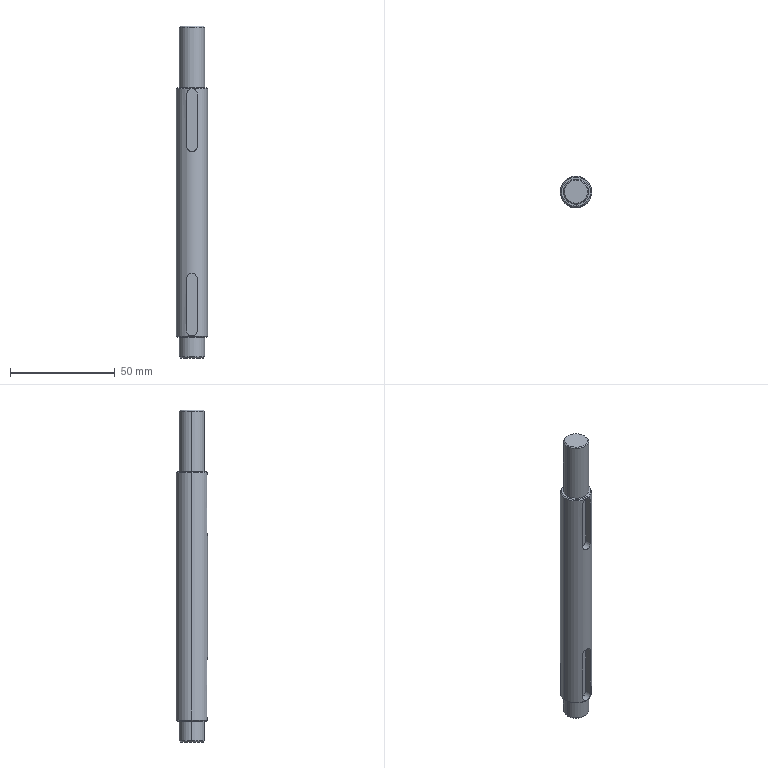Part | SolidWorks | features ICE 3, Chamfer 2, Extrusion 1 | 1 solid | 30 faces | box 15 x 15 x 158.5 mm | volume 24503 mm3 | cylinder 12 | plane 10 | cone 8 | commonest cylinder face diameters 5 x6 12 x4 15 x2
STEP:
#1=CARTESIAN_POINT('',(2.5,-7.071,-120.5));
#2=VERTEX_POINT('',#1);
#3=CARTESIAN_POINT('',(0.,-7.5,-118.));
#4=VERTEX_POINT('',#3);
#5=CARTESIAN_POINT('',(2.5,-7.071,-120.5));
#6=CARTESIAN_POINT('',(2.5,-7.071,-120.335));
#7=CARTESIAN_POINT('',(2.484,-7.077,-120.172));
#8=CARTESIAN_POINT('',(2.419,-7.099,-119.849));
#9=CARTESIAN_POINT('',(2.371,-7.116,-119.69));
#10=CARTESIAN_POINT('',(2.183,-7.177,-119.238));
#11=CARTESIAN_POINT('',(1.997,-7.233,-118.962));
#12=CARTESIAN_POINT('',(1.654,-7.316,-118.618));
#13=CARTESIAN_POINT('',(1.526,-7.344,-118.513));
#14=CARTESIAN_POINT('',(1.256,-7.395,-118.332));
#15=CARTESIAN_POINT('',(1.113,-7.419,-118.255));
#16=CARTESIAN_POINT('',(0.8106,-7.458,-118.129));
#17=CARTESIAN_POINT('',(0.6511,-7.473,-118.081));
#18=CARTESIAN_POINT('',(0.33,-7.494,-118.016));
#19=CARTESIAN_POINT('',(0.1664,-7.5,-118.));
#20=CARTESIAN_POINT('',(0.,-7.5,-118.));
#21=B_SPLINE_CURVE_WITH_KNOTS('',3,(#5,#6,#7,#8,#9,#10,#11,#12,#13,#14,#15,#16,#17,#18,#19,#20),.UNSPECIFIED.,.F.,.F.,(4,2,2,2,2,2,2,4),(0.01181,0.0123,0.01279,0.01378,0.01427,0.01476,0.01525,0.01574),.UNSPECIFIED.);
#22=EDGE_CURVE('',#2,#4,#21,.T.);
#23=ORIENTED_EDGE('',*,*,#22,.T.);
#24=CARTESIAN_POINT('',(0.,-4.,-118.));
#25=VERTEX_POINT('',#24);
#26=CARTESIAN_POINT('',(0.,-52.,-118.));
#27=DIRECTION('',(0.,1.,0.));
#28=VECTOR('',#27,1000.);
#29=LINE('',#26,#28);
#30=EDGE_CURVE('',#4,#25,#29,.T.);
#31=ORIENTED_EDGE('',*,*,#30,.T.);
#32=CARTESIAN_POINT('',(2.5,-4.,-120.5));
#33=VERTEX_POINT('',#32);
#34=CARTESIAN_POINT('',(0.,-4.,-120.5));
#35=DIRECTION('',(0.,1.,0.));
#36=DIRECTION('',(0.,0.,1.));
#37=AXIS2_PLACEMENT_3D('',#34,#35,#36);
#38=CIRCLE('',#37,2.5);
#39=EDGE_CURVE('',#25,#33,#38,.T.);
#40=ORIENTED_EDGE('',*,*,#39,.T.);
#41=CARTESIAN_POINT('',(2.5,-52.,-120.5));
#42=DIRECTION('',(0.,1.,0.));
#43=VECTOR('',#42,1000.);
#44=LINE('',#41,#43);
#45=EDGE_CURVE('',#2,#33,#44,.T.);
#46=ORIENTED_EDGE('',*,*,#45,.F.);
#47=EDGE_LOOP('',(#23,#31,#40,#46));
#48=FACE_OUTER_BOUND('',#47,.T.);
#49=CARTESIAN_POINT('',(0.,-52.,-120.5));
#50=DIRECTION('',(0.,1.,0.));
#51=DIRECTION('',(0.,0.,1.));
#52=AXIS2_PLACEMENT_3D('',#49,#50,#51);
#53=CYLINDRICAL_SURFACE('',#52,2.5);
#54=ADVANCED_FACE('',(#48),#53,.F.);
#55=CARTESIAN_POINT('',(2.5,-7.071,-32.5));
#56=VERTEX_POINT('',#55);
#57=CARTESIAN_POINT('',(0.,-7.5,-30.));
#58=VERTEX_POINT('',#57);
#59=CARTESIAN_POINT('',(2.5,-7.071,-32.5));
#60=CARTESIAN_POINT('',(2.5,-7.071,-32.335));
#61=CARTESIAN_POINT('',(2.484,-7.077,-32.172));
#62=CARTESIAN_POINT('',(2.419,-7.099,-31.849));
#63=CARTESIAN_POINT('',(2.371,-7.116,-31.69));
#64=CARTESIAN_POINT('',(2.183,-7.177,-31.238));
#65=CARTESIAN_POINT('',(1.997,-7.233,-30.962));
#66=CARTESIAN_POINT('',(1.654,-7.316,-30.618));
#67=CARTESIAN_POINT('',(1.526,-7.344,-30.513));
#68=CARTESIAN_POINT('',(1.256,-7.395,-30.332));
#69=CARTESIAN_POINT('',(1.113,-7.419,-30.255));
#70=CARTESIAN_POINT('',(0.8106,-7.458,-30.129));
#71=CARTESIAN_POINT('',(0.6511,-7.473,-30.081));
#72=CARTESIAN_POINT('',(0.33,-7.494,-30.016));
#73=CARTESIAN_POINT('',(0.1664,-7.5,-30.));
#74=CARTESIAN_POINT('',(0.,-7.5,-30.));
#75=B_SPLINE_CURVE_WITH_KNOTS('',3,(#59,#60,#61,#62,#63,#64,#65,#66,#67,#68,#69,#70,#71,#72,#73,#74),.UNSPECIFIED.,.F.,.F.,(4,2,2,2,2,2,2,4),(0.01181,0.0123,0.01279,0.01378,0.01427,0.01476,0.01525,0.01574),.UNSPECIFIED.);
#76=EDGE_CURVE('',#56,#58,#75,.T.);
#77=ORIENTED_EDGE('',*,*,#76,.T.);
#78=CARTESIAN_POINT('',(0.,-4.,-30.));
#79=VERTEX_POINT('',#78);
#80=CARTESIAN_POINT('',(0.,-52.,-30.));
#81=DIRECTION('',(0.,1.,0.));
#82=VECTOR('',#81,1000.);
#83=LINE('',#80,#82);
#84=EDGE_CURVE('',#58,#79,#83,.T.);
#85=ORIENTED_EDGE('',*,*,#84,.T.);
#86=CARTESIAN_POINT('',(2.5,-4.,-32.5));
#87=VERTEX_POINT('',#86);
#88=CARTESIAN_POINT('',(0.,-4.,-32.5));
#89=DIRECTION('',(0.,1.,0.));
#90=DIRECTION('',(0.,0.,1.));
#91=AXIS2_PLACEMENT_3D('',#88,#89,#90);
#92=CIRCLE('',#91,2.5);
#93=EDGE_CURVE('',#79,#87,#92,.T.);
#94=ORIENTED_EDGE('',*,*,#93,.T.);
#95=CARTESIAN_POINT('',(2.5,-52.,-32.5));
#96=DIRECTION('',(0.,1.,0.));
#97=VECTOR('',#96,1000.);
#98=LINE('',#95,#97);
#99=EDGE_CURVE('',#56,#87,#98,.T.);
#100=ORIENTED_EDGE('',*,*,#99,.F.);
#101=EDGE_LOOP('',(#77,#85,#94,#100));
#102=FACE_OUTER_BOUND('',#101,.T.);
#103=CARTESIAN_POINT('',(0.,-52.,-32.5));
#104=DIRECTION('',(0.,1.,0.));
#105=DIRECTION('',(0.,0.,1.));
#106=AXIS2_PLACEMENT_3D('',#103,#104,#105);
#107=CYLINDRICAL_SURFACE('',#106,2.5);
#108=ADVANCED_FACE('',(#102),#107,.F.);
#109=CARTESIAN_POINT('',(-5.5,0.,-158.5));
#110=VERTEX_POINT('',#109);
#111=CARTESIAN_POINT('',(5.5,0.,-158.5));
#112=VERTEX_POINT('',#111);
#113=CARTESIAN_POINT('',(0.,0.,-158.5));
#114=DIRECTION('',(0.,0.,-1.));
#115=DIRECTION('',(1.,0.,0.));
#116=AXIS2_PLACEMENT_3D('',#113,#114,#115);
#117=CIRCLE('',#116,5.5);
#118=EDGE_CURVE('',#110,#112,#117,.T.);
#119=ORIENTED_EDGE('',*,*,#118,.F.);
#120=CARTESIAN_POINT('',(-6.,0.,-158.));
#121=VERTEX_POINT('',#120);
#122=CARTESIAN_POINT('',(-5.5,0.,-158.5));
#123=DIRECTION('',(-0.7071,0.,0.7071));
#124=VECTOR('',#123,1000.);
#125=LINE('',#122,#124);
#126=EDGE_CURVE('',#110,#121,#125,.T.);
#127=ORIENTED_EDGE('',*,*,#126,.T.);
#128=CARTESIAN_POINT('',(6.,0.,-158.));
#129=VERTEX_POINT('',#128);
#130=CARTESIAN_POINT('',(0.,0.,-158.));
#131=DIRECTION('',(0.,0.,1.));
#132=DIRECTION('',(1.,0.,0.));
#133=AXIS2_PLACEMENT_3D('',#130,#131,#132);
#134=CIRCLE('',#133,6.);
#135=EDGE_CURVE('',#129,#121,#134,.T.);
#136=ORIENTED_EDGE('',*,*,#135,.F.);
#137=CARTESIAN_POINT('',(5.5,0.,-158.5));
#138=DIRECTION('',(0.7071,0.,0.7071));
#139=VECTOR('',#138,1000.);
#140=LINE('',#137,#139);
#141=EDGE_CURVE('',#112,#129,#140,.T.);
#142=ORIENTED_EDGE('',*,*,#141,.F.);
#143=EDGE_LOOP('',(#119,#127,#136,#142));
#144=FACE_OUTER_BOUND('',#143,.T.);
#145=CARTESIAN_POINT('',(0.,0.,-158.5));
#146=DIRECTION('',(0.,0.,1.));
#147=DIRECTION('',(1.,0.,0.));
#148=AXIS2_PLACEMENT_3D('',#145,#146,#147);
#149=CONICAL_SURFACE('',#148,5.5,0.7854);
#150=ADVANCED_FACE('',(#144),#149,.T.);
#151=CARTESIAN_POINT('',(-7.,0.,-148.5));
#152=VERTEX_POINT('',#151);
#153=CARTESIAN_POINT('',(7.,0.,-148.5));
#154=VERTEX_POINT('',#153);
#155=CARTESIAN_POINT('',(0.,0.,-148.5));
#156=DIRECTION('',(0.,0.,-1.));
#157=DIRECTION('',(-1.,0.,0.));
#158=AXIS2_PLACEMENT_3D('',#155,#156,#157);
#159=CIRCLE('',#158,7.);
#160=EDGE_CURVE('',#152,#154,#159,.T.);
#161=ORIENTED_EDGE('',*,*,#160,.F.);
#162=CARTESIAN_POINT('',(-7.5,0.,-148.));
#163=VERTEX_POINT('',#162);
#164=CARTESIAN_POINT('',(-7.5,0.,-148.));
#165=DIRECTION('',(-0.7071,0.,0.7071));
#166=VECTOR('',#165,1000.);
#167=LINE('',#164,#166);
#168=EDGE_CURVE('',#152,#163,#167,.T.);
#169=ORIENTED_EDGE('',*,*,#168,.T.);
#170=CARTESIAN_POINT('',(7.5,0.,-148.));
#171=VERTEX_POINT('',#170);
#172=CARTESIAN_POINT('',(0.,0.,-148.));
#173=DIRECTION('',(0.,0.,1.));
#174=DIRECTION('',(-1.,0.,0.));
#175=AXIS2_PLACEMENT_3D('',#172,#173,#174);
#176=CIRCLE('',#175,7.5);
#177=EDGE_CURVE('',#171,#163,#176,.T.);
#178=ORIENTED_EDGE('',*,*,#177,.F.);
#179=CARTESIAN_POINT('',(7.5,0.,-148.));
#180=DIRECTION('',(0.7071,0.,0.7071));
#181=VECTOR('',#180,1000.);
#182=LINE('',#179,#181);
#183=EDGE_CURVE('',#154,#171,#182,.T.);
#184=ORIENTED_EDGE('',*,*,#183,.F.);
#185=EDGE_LOOP('',(#161,#169,#178,#184));
#186=FACE_OUTER_BOUND('',#185,.T.);
#187=CARTESIAN_POINT('',(0.,0.,-148.));
#188=DIRECTION('',(0.,0.,1.));
#189=DIRECTION('',(1.,0.,0.));
#190=AXIS2_PLACEMENT_3D('',#187,#188,#189);
#191=CONICAL_SURFACE('',#190,7.5,0.7854);
#192=ADVANCED_FACE('',(#186),#191,.T.);
#193=CARTESIAN_POINT('',(-6.,0.,-148.5));
#194=VERTEX_POINT('',#193);
#195=CARTESIAN_POINT('',(6.,0.,-148.5));
#196=VERTEX_POINT('',#195);
#197=CARTESIAN_POINT('',(0.,0.,-148.5));
#198=DIRECTION('',(0.,0.,-1.));
#199=DIRECTION('',(-1.,0.,0.));
#200=AXIS2_PLACEMENT_3D('',#197,#198,#199);
#201=CIRCLE('',#200,6.);
#202=EDGE_CURVE('',#194,#196,#201,.T.);
#203=ORIENTED_EDGE('',*,*,#202,.T.);
#204=CARTESIAN_POINT('',(6.,0.,-148.5));
#205=DIRECTION('',(0.,0.,-1.));
#206=VECTOR('',#205,1000.);
#207=LINE('',#204,#206);
#208=EDGE_CURVE('',#196,#129,#207,.T.);
#209=ORIENTED_EDGE('',*,*,#208,.T.);
#210=ORIENTED_EDGE('',*,*,#135,.T.);
#211=CARTESIAN_POINT('',(-6.,0.,-148.5));
#212=DIRECTION('',(0.,0.,-1.));
#213=VECTOR('',#212,1000.);
#214=LINE('',#211,#213);
#215=EDGE_CURVE('',#194,#121,#214,.T.);
#216=ORIENTED_EDGE('',*,*,#215,.F.);
#217=EDGE_LOOP('',(#203,#209,#210,#216));
#218=FACE_OUTER_BOUND('',#217,.T.);
#219=CARTESIAN_POINT('',(0.,0.,-148.5));
#220=DIRECTION('',(0.,0.,-1.));
#221=DIRECTION('',(-1.,0.,0.));
#222=AXIS2_PLACEMENT_3D('',#219,#220,#221);
#223=CYLINDRICAL_SURFACE('',#222,6.);
#224=ADVANCED_FACE('',(#218),#223,.T.);
#225=CARTESIAN_POINT('',(5.5,0.,0.));
#226=VERTEX_POINT('',#225);
#227=CARTESIAN_POINT('',(-5.5,0.,0.));
#228=VERTEX_POINT('',#227);
#229=CARTESIAN_POINT('',(0.,0.,0.));
#230=DIRECTION('',(0.,0.,1.));
#231=DIRECTION('',(1.,0.,0.));
#232=AXIS2_PLACEMENT_3D('',#229,#230,#231);
#233=CIRCLE('',#232,5.5);
#234=EDGE_CURVE('',#226,#228,#233,.T.);
#235=ORIENTED_EDGE('',*,*,#234,.F.);
#236=CARTESIAN_POINT('',(6.,0.,-0.5));
#237=VERTEX_POINT('',#236);
#238=CARTESIAN_POINT('',(5.5,0.,0.));
#239=DIRECTION('',(0.7071,0.,-0.7071));
#240=VECTOR('',#239,1000.);
#241=LINE('',#238,#240);
#242=EDGE_CURVE('',#226,#237,#241,.T.);
#243=ORIENTED_EDGE('',*,*,#242,.T.);
#244=CARTESIAN_POINT('',(-6.,0.,-0.5));
#245=VERTEX_POINT('',#244);
#246=CARTESIAN_POINT('',(0.,0.,-0.5));
#247=DIRECTION('',(0.,0.,-1.));
#248=DIRECTION('',(1.,0.,0.));
#249=AXIS2_PLACEMENT_3D('',#246,#247,#248);
#250=CIRCLE('',#249,6.);
#251=EDGE_CURVE('',#245,#237,#250,.T.);
#252=ORIENTED_EDGE('',*,*,#251,.F.);
#253=CARTESIAN_POINT('',(-5.5,0.,0.));
#254=DIRECTION('',(-0.7071,0.,-0.7071));
#255=VECTOR('',#254,1000.);
#256=LINE('',#253,#255);
#257=EDGE_CURVE('',#228,#245,#256,.T.);
#258=ORIENTED_EDGE('',*,*,#257,.F.);
#259=EDGE_LOOP('',(#235,#243,#252,#258));
#260=FACE_OUTER_BOUND('',#259,.T.);
#261=CARTESIAN_POINT('',(0.,0.,0.));
#262=DIRECTION('',(0.,0.,-1.));
#263=DIRECTION('',(-1.,0.,0.));
#264=AXIS2_PLACEMENT_3D('',#261,#262,#263);
#265=CONICAL_SURFACE('',#264,5.5,0.7854);
#266=ADVANCED_FACE('',(#260),#265,.T.);
#267=CARTESIAN_POINT('',(7.,0.,-29.5));
#268=VERTEX_POINT('',#267);
#269=CARTESIAN_POINT('',(-7.,0.,-29.5));
#270=VERTEX_POINT('',#269);
#271=CARTESIAN_POINT('',(0.,0.,-29.5));
#272=DIRECTION('',(0.,0.,1.));
#273=DIRECTION('',(1.,0.,0.));
#274=AXIS2_PLACEMENT_3D('',#271,#272,#273);
#275=CIRCLE('',#274,7.);
#276=EDGE_CURVE('',#268,#270,#275,.T.);
#277=ORIENTED_EDGE('',*,*,#276,.F.);
#278=CARTESIAN_POINT('',(7.5,0.,-30.));
#279=VERTEX_POINT('',#278);
#280=CARTESIAN_POINT('',(7.5,0.,-30.));
#281=DIRECTION('',(0.7071,0.,-0.7071));
#282=VECTOR('',#281,1000.);
#283=LINE('',#280,#282);
#284=EDGE_CURVE('',#268,#279,#283,.T.);
#285=ORIENTED_EDGE('',*,*,#284,.T.);
#286=CARTESIAN_POINT('',(-7.5,0.,-30.));
#287=VERTEX_POINT('',#286);
#288=CARTESIAN_POINT('',(0.,0.,-30.));
#289=DIRECTION('',(0.,0.,-1.));
#290=DIRECTION('',(1.,0.,0.));
#291=AXIS2_PLACEMENT_3D('',#288,#289,#290);
#292=CIRCLE('',#291,7.5);
#293=EDGE_CURVE('',#287,#279,#292,.T.);
#294=ORIENTED_EDGE('',*,*,#293,.F.);
#295=CARTESIAN_POINT('',(-7.5,0.,-30.));
#296=DIRECTION('',(-0.7071,0.,-0.7071));
#297=VECTOR('',#296,1000.);
#298=LINE('',#295,#297);
#299=EDGE_CURVE('',#270,#287,#298,.T.);
#300=ORIENTED_EDGE('',*,*,#299,.F.);
#301=EDGE_LOOP('',(#277,#285,#294,#300));
#302=FACE_OUTER_BOUND('',#301,.T.);
#303=CARTESIAN_POINT('',(0.,0.,-30.));
#304=DIRECTION('',(0.,0.,-1.));
#305=DIRECTION('',(-1.,0.,0.));
#306=AXIS2_PLACEMENT_3D('',#303,#304,#305);
#307=CONICAL_SURFACE('',#306,7.5,0.7854);
#308=ADVANCED_FACE('',(#302),#307,.T.);
#309=CARTESIAN_POINT('',(6.,0.,-29.5));
#310=VERTEX_POINT('',#309);
#311=CARTESIAN_POINT('',(-6.,0.,-29.5));
#312=VERTEX_POINT('',#311);
#313=CARTESIAN_POINT('',(0.,0.,-29.5));
#314=DIRECTION('',(0.,0.,1.));
#315=DIRECTION('',(1.,0.,0.));
#316=AXIS2_PLACEMENT_3D('',#313,#314,#315);
#317=CIRCLE('',#316,6.);
#318=EDGE_CURVE('',#310,#312,#317,.T.);
#319=ORIENTED_EDGE('',*,*,#318,.T.);
#320=CARTESIAN_POINT('',(-6.,0.,-29.5));
#321=DIRECTION('',(0.,0.,1.));
#322=VECTOR('',#321,1000.);
#323=LINE('',#320,#322);
#324=EDGE_CURVE('',#312,#245,#323,.T.);
#325=ORIENTED_EDGE('',*,*,#324,.T.);
#326=ORIENTED_EDGE('',*,*,#251,.T.);
#327=CARTESIAN_POINT('',(6.,0.,-29.5));
#328=DIRECTION('',(0.,0.,1.));
#329=VECTOR('',#328,1000.);
#330=LINE('',#327,#329);
#331=EDGE_CURVE('',#310,#237,#330,.T.);
#332=ORIENTED_EDGE('',*,*,#331,.F.);
#333=EDGE_LOOP('',(#319,#325,#326,#332));
#334=FACE_OUTER_BOUND('',#333,.T.);
#335=CARTESIAN_POINT('',(0.,0.,-29.5));
#336=DIRECTION('',(0.,0.,1.));
#337=DIRECTION('',(1.,0.,0.));
#338=AXIS2_PLACEMENT_3D('',#335,#336,#337);
#339=CYLINDRICAL_SURFACE('',#338,6.);
#340=ADVANCED_FACE('',(#334),#339,.T.);
#341=ORIENTED_EDGE('',*,*,#177,.T.);
#342=CARTESIAN_POINT('',(-7.5,0.,-158.5));
#343=DIRECTION('',(0.,0.,1.));
#344=VECTOR('',#343,1000.);
#345=LINE('',#342,#344);
#346=EDGE_CURVE('',#163,#287,#345,.T.);
#347=ORIENTED_EDGE('',*,*,#346,.T.);
#348=ORIENTED_EDGE('',*,*,#293,.T.);
#349=CARTESIAN_POINT('',(7.5,0.,-158.5));
#350=DIRECTION('',(0.,0.,1.));
#351=VECTOR('',#350,1000.);
#352=LINE('',#349,#351);
#353=EDGE_CURVE('',#171,#279,#352,.T.);
#354=ORIENTED_EDGE('',*,*,#353,.F.);
#355=EDGE_LOOP('',(#341,#347,#348,#354));
#356=FACE_OUTER_BOUND('',#355,.T.);
#357=CARTESIAN_POINT('',(0.,0.,-158.5));
#358=DIRECTION('',(0.,0.,1.));
#359=DIRECTION('',(1.,0.,0.));
#360=AXIS2_PLACEMENT_3D('',#357,#358,#359);
#361=CYLINDRICAL_SURFACE('',#360,7.5);
#362=ADVANCED_FACE('',(#356),#361,.T.);
#363=ORIENTED_EDGE('',*,*,#346,.F.);
#364=CARTESIAN_POINT('',(0.,-7.5,-148.));
#365=VERTEX_POINT('',#364);
#366=CARTESIAN_POINT('',(0.,0.,-148.));
#367=DIRECTION('',(0.,0.,1.));
#368=DIRECTION('',(-1.,0.,0.));
#369=AXIS2_PLACEMENT_3D('',#366,#367,#368);
#370=CIRCLE('',#369,7.5);
#371=EDGE_CURVE('',#163,#365,#370,.T.);
#372=ORIENTED_EDGE('',*,*,#371,.T.);
#373=CARTESIAN_POINT('',(-2.5,-7.071,-145.5));
#374=VERTEX_POINT('',#373);
#375=CARTESIAN_POINT('',(-2.5,-7.071,-145.5));
#376=CARTESIAN_POINT('',(-2.5,-7.071,-145.664));
#377=CARTESIAN_POINT('',(-2.483,-7.077,-145.831));
#378=CARTESIAN_POINT('',(-2.419,-7.099,-146.153));
#379=CARTESIAN_POINT('',(-2.371,-7.116,-146.309));
#380=CARTESIAN_POINT('',(-2.244,-7.157,-146.613));
#381=CARTESIAN_POINT('',(-2.167,-7.181,-146.757));
#382=CARTESIAN_POINT('',(-1.986,-7.233,-147.027));
#383=CARTESIAN_POINT('',(-1.882,-7.261,-147.154));
#384=CARTESIAN_POINT('',(-1.652,-7.317,-147.384));
#385=CARTESIAN_POINT('',(-1.527,-7.344,-147.486));
#386=CARTESIAN_POINT('',(-1.257,-7.395,-147.667));
#387=CARTESIAN_POINT('',(-1.11,-7.419,-147.746));
#388=CARTESIAN_POINT('',(-0.8092,-7.458,-147.871));
#389=CARTESIAN_POINT('',(-0.6532,-7.473,-147.919));
#390=CARTESIAN_POINT('',(-0.3296,-7.495,-147.984));
#391=CARTESIAN_POINT('',(-0.1639,-7.5,-148.));
#392=CARTESIAN_POINT('',(0.,-7.5,-148.));
#393=B_SPLINE_CURVE_WITH_KNOTS('',3,(#375,#376,#377,#378,#379,#380,#381,#382,#383,#384,#385,#386,#387,#388,#389,#390,#391,#392),.UNSPECIFIED.,.F.,.F.,(4,2,2,2,2,2,2,2,4),(0.003938,0.00443,0.004921,0.005413,0.005905,0.006397,0.006889,0.007381,0.007873),.UNSPECIFIED.);
#394=EDGE_CURVE('',#374,#365,#393,.T.);
#395=ORIENTED_EDGE('',*,*,#394,.F.);
#396=CARTESIAN_POINT('',(-2.5,-7.071,-120.5));
#397=VERTEX_POINT('',#396);
#398=CARTESIAN_POINT('',(-2.5,-7.071,-158.5));
#399=DIRECTION('',(0.,0.,-1.));
#400=VECTOR('',#399,1000.);
#401=LINE('',#398,#400);
#402=EDGE_CURVE('',#397,#374,#401,.T.);
#403=ORIENTED_EDGE('',*,*,#402,.F.);
#404=CARTESIAN_POINT('',(0.,-7.5,-118.));
#405=CARTESIAN_POINT('',(-0.1665,-7.5,-118.));
#406=CARTESIAN_POINT('',(-0.33,-7.494,-118.016));
#407=CARTESIAN_POINT('',(-0.6513,-7.473,-118.081));
#408=CARTESIAN_POINT('',(-0.8108,-7.458,-118.129));
#409=CARTESIAN_POINT('',(-1.113,-7.418,-118.256));
#410=CARTESIAN_POINT('',(-1.256,-7.395,-118.333));
#411=CARTESIAN_POINT('',(-1.527,-7.344,-118.514));
#412=CARTESIAN_POINT('',(-1.655,-7.316,-118.619));
#413=CARTESIAN_POINT('',(-1.998,-7.233,-118.963));
#414=CARTESIAN_POINT('',(-2.183,-7.176,-119.24));
#415=CARTESIAN_POINT('',(-2.371,-7.116,-119.69));
#416=CARTESIAN_POINT('',(-2.419,-7.099,-119.849));
#417=CARTESIAN_POINT('',(-2.484,-7.077,-120.172));
#418=CARTESIAN_POINT('',(-2.5,-7.071,-120.336));
#419=CARTESIAN_POINT('',(-2.5,-7.071,-120.5));
#420=B_SPLINE_CURVE_WITH_KNOTS('',3,(#404,#405,#406,#407,#408,#409,#410,#411,#412,#413,#414,#415,#416,#417,#418,#419),.UNSPECIFIED.,.F.,.F.,(4,2,2,2,2,2,2,4),(0.,0.0004922,0.0009844,0.001477,0.001969,0.002953,0.003445,0.003938),.UNSPECIFIED.);
#421=EDGE_CURVE('',#4,#397,#420,.T.);
#422=ORIENTED_EDGE('',*,*,#421,.F.);
#423=ORIENTED_EDGE('',*,*,#22,.F.);
#424=CARTESIAN_POINT('',(2.5,-7.071,-145.5));
#425=VERTEX_POINT('',#424);
#426=CARTESIAN_POINT('',(2.5,-7.071,-158.5));
#427=DIRECTION('',(0.,0.,1.));
#428=VECTOR('',#427,1000.);
#429=LINE('',#426,#428);
#430=EDGE_CURVE('',#425,#2,#429,.T.);
#431=ORIENTED_EDGE('',*,*,#430,.F.);
#432=CARTESIAN_POINT('',(0.,-7.5,-148.));
#433=CARTESIAN_POINT('',(0.1639,-7.5,-148.));
#434=CARTESIAN_POINT('',(0.329,-7.495,-147.984));
#435=CARTESIAN_POINT('',(0.6533,-7.473,-147.919));
#436=CARTESIAN_POINT('',(0.8096,-7.458,-147.871));
#437=CARTESIAN_POINT('',(1.111,-7.419,-147.745));
#438=CARTESIAN_POINT('',(1.258,-7.395,-147.667));
#439=CARTESIAN_POINT('',(1.527,-7.344,-147.486));
#440=CARTESIAN_POINT('',(1.653,-7.317,-147.383));
#441=CARTESIAN_POINT('',(1.999,-7.233,-147.037));
#442=CARTESIAN_POINT('',(2.182,-7.177,-146.764));
#443=CARTESIAN_POINT('',(2.371,-7.116,-146.308));
#444=CARTESIAN_POINT('',(2.419,-7.099,-146.152));
#445=CARTESIAN_POINT('',(2.483,-7.077,-145.831));
#446=CARTESIAN_POINT('',(2.5,-7.071,-145.665));
#447=CARTESIAN_POINT('',(2.5,-7.071,-145.5));
#448=B_SPLINE_CURVE_WITH_KNOTS('',3,(#432,#433,#434,#435,#436,#437,#438,#439,#440,#441,#442,#443,#444,#445,#446,#447),.UNSPECIFIED.,.F.,.F.,(4,2,2,2,2,2,2,4),(0.007873,0.008365,0.008857,0.009349,0.00984,0.01082,0.01132,0.01181),.UNSPECIFIED.);
#449=EDGE_CURVE('',#365,#425,#448,.T.);
#450=ORIENTED_EDGE('',*,*,#449,.F.);
#451=CARTESIAN_POINT('',(0.,0.,-148.));
#452=DIRECTION('',(0.,0.,1.));
#453=DIRECTION('',(-1.,0.,0.));
#454=AXIS2_PLACEMENT_3D('',#451,#452,#453);
#455=CIRCLE('',#454,7.5);
#456=EDGE_CURVE('',#365,#171,#455,.T.);
#457=ORIENTED_EDGE('',*,*,#456,.T.);
#458=ORIENTED_EDGE('',*,*,#353,.T.);
#459=CARTESIAN_POINT('',(0.,0.,-30.));
#460=DIRECTION('',(0.,0.,-1.));
#461=DIRECTION('',(1.,0.,0.));
#462=AXIS2_PLACEMENT_3D('',#459,#460,#461);
#463=CIRCLE('',#462,7.5);
#464=EDGE_CURVE('',#279,#58,#463,.T.);
#465=ORIENTED_EDGE('',*,*,#464,.T.);
#466=ORIENTED_EDGE('',*,*,#76,.F.);
#467=CARTESIAN_POINT('',(2.5,-7.071,-57.5));
#468=VERTEX_POINT('',#467);
#469=CARTESIAN_POINT('',(2.5,-7.071,-158.5));
#470=DIRECTION('',(0.,0.,1.));
#471=VECTOR('',#470,1000.);
#472=LINE('',#469,#471);
#473=EDGE_CURVE('',#468,#56,#472,.T.);
#474=ORIENTED_EDGE('',*,*,#473,.F.);
#475=CARTESIAN_POINT('',(-2.5,-7.071,-57.5));
#476=VERTEX_POINT('',#475);
#477=CARTESIAN_POINT('',(-2.5,-7.071,-57.5));
#478=CARTESIAN_POINT('',(-2.5,-7.071,-57.664));
#479=CARTESIAN_POINT('',(-2.483,-7.077,-57.831));
#480=CARTESIAN_POINT('',(-2.419,-7.099,-58.153));
#481=CARTESIAN_POINT('',(-2.371,-7.116,-58.309));
#482=CARTESIAN_POINT('',(-2.244,-7.157,-58.613));
#483=CARTESIAN_POINT('',(-2.167,-7.181,-58.757));
#484=CARTESIAN_POINT('',(-1.986,-7.233,-59.027));
#485=CARTESIAN_POINT('',(-1.882,-7.261,-59.154));
#486=CARTESIAN_POINT('',(-1.652,-7.317,-59.384));
#487=CARTESIAN_POINT('',(-1.527,-7.344,-59.486));
#488=CARTESIAN_POINT('',(-1.257,-7.395,-59.667));
#489=CARTESIAN_POINT('',(-1.11,-7.419,-59.746));
#490=CARTESIAN_POINT('',(-0.8093,-7.458,-59.871));
#491=CARTESIAN_POINT('',(-0.6533,-7.473,-59.919));
#492=CARTESIAN_POINT('',(-0.3296,-7.495,-59.984));
#493=CARTESIAN_POINT('',(-0.164,-7.5,-60.));
#494=CARTESIAN_POINT('',(0.1639,-7.5,-60.));
#495=CARTESIAN_POINT('',(0.329,-7.495,-59.984));
#496=CARTESIAN_POINT('',(0.6533,-7.473,-59.919));
#497=CARTESIAN_POINT('',(0.8096,-7.458,-59.871));
#498=CARTESIAN_POINT('',(1.111,-7.419,-59.745));
#499=CARTESIAN_POINT('',(1.257,-7.395,-59.667));
#500=CARTESIAN_POINT('',(1.527,-7.344,-59.486));
#501=CARTESIAN_POINT('',(1.653,-7.317,-59.383));
#502=CARTESIAN_POINT('',(1.999,-7.233,-59.037));
#503=CARTESIAN_POINT('',(2.182,-7.177,-58.764));
#504=CARTESIAN_POINT('',(2.371,-7.116,-58.308));
#505=CARTESIAN_POINT('',(2.419,-7.099,-58.152));
#506=CARTESIAN_POINT('',(2.483,-7.077,-57.831));
#507=CARTESIAN_POINT('',(2.5,-7.071,-57.665));
#508=CARTESIAN_POINT('',(2.5,-7.071,-57.5));
#509=B_SPLINE_CURVE_WITH_KNOTS('',3,(#477,#478,#479,#480,#481,#482,#483,#484,#485,#486,#487,#488,#489,#490,#491,#492,#493,#494,#495,#496,#497,#498,#499,#500,#501,#502,#503,#504,#505,#506,#507,#508),.UNSPECIFIED.,.F.,.F.,(4,2,2,2,2,2,2,2,2,2,2,2,2,2,2,4),(0.003938,0.00443,0.004921,0.005413,0.005905,0.006397,0.006889,0.007381,0.007873,0.008365,0.008857,0.009349,0.00984,0.01082,0.01132,0.01181),.UNSPECIFIED.);
#510=EDGE_CURVE('',#476,#468,#509,.T.);
#511=ORIENTED_EDGE('',*,*,#510,.F.);
#512=CARTESIAN_POINT('',(-2.5,-7.071,-32.5));
#513=VERTEX_POINT('',#512);
#514=CARTESIAN_POINT('',(-2.5,-7.071,-158.5));
#515=DIRECTION('',(0.,0.,-1.));
#516=VECTOR('',#515,1000.);
#517=LINE('',#514,#516);
#518=EDGE_CURVE('',#513,#476,#517,.T.);
#519=ORIENTED_EDGE('',*,*,#518,.F.);
#520=CARTESIAN_POINT('',(0.,-7.5,-30.));
#521=CARTESIAN_POINT('',(-0.1665,-7.5,-30.));
#522=CARTESIAN_POINT('',(-0.33,-7.494,-30.016));
#523=CARTESIAN_POINT('',(-0.6513,-7.473,-30.081));
#524=CARTESIAN_POINT('',(-0.8108,-7.458,-30.129));
#525=CARTESIAN_POINT('',(-1.113,-7.418,-30.256));
#526=CARTESIAN_POINT('',(-1.256,-7.395,-30.333));
#527=CARTESIAN_POINT('',(-1.527,-7.344,-30.514));
#528=CARTESIAN_POINT('',(-1.655,-7.316,-30.619));
#529=CARTESIAN_POINT('',(-1.998,-7.233,-30.963));
#530=CARTESIAN_POINT('',(-2.183,-7.176,-31.24));
#531=CARTESIAN_POINT('',(-2.371,-7.116,-31.69));
#532=CARTESIAN_POINT('',(-2.419,-7.099,-31.849));
#533=CARTESIAN_POINT('',(-2.484,-7.077,-32.172));
#534=CARTESIAN_POINT('',(-2.5,-7.071,-32.336));
#535=CARTESIAN_POINT('',(-2.5,-7.071,-32.5));
#536=B_SPLINE_CURVE_WITH_KNOTS('',3,(#520,#521,#522,#523,#524,#525,#526,#527,#528,#529,#530,#531,#532,#533,#534,#535),.UNSPECIFIED.,.F.,.F.,(4,2,2,2,2,2,2,4),(0.,0.0004922,0.0009844,0.001477,0.001969,0.002953,0.003445,0.003938),.UNSPECIFIED.);
#537=EDGE_CURVE('',#58,#513,#536,.T.);
#538=ORIENTED_EDGE('',*,*,#537,.F.);
#539=CARTESIAN_POINT('',(0.,0.,-30.));
#540=DIRECTION('',(0.,0.,-1.));
#541=DIRECTION('',(1.,0.,0.));
#542=AXIS2_PLACEMENT_3D('',#539,#540,#541);
#543=CIRCLE('',#542,7.5);
#544=EDGE_CURVE('',#58,#287,#543,.T.);
#545=ORIENTED_EDGE('',*,*,#544,.T.);
#546=EDGE_LOOP('',(#363,#372,#395,#403,#422,#423,#431,#450,#457,#458,#465,#466,#474,#511,#519,#538,#545));
#547=FACE_OUTER_BOUND('',#546,.T.);
#548=CARTESIAN_POINT('',(0.,0.,-158.5));
#549=DIRECTION('',(0.,0.,1.));
#550=DIRECTION('',(1.,0.,0.));
#551=AXIS2_PLACEMENT_3D('',#548,#549,#550);
#552=CYLINDRICAL_SURFACE('',#551,7.5);
#553=ADVANCED_FACE('',(#547),#552,.T.);
#554=CARTESIAN_POINT('',(0.,0.,-29.5));
#555=DIRECTION('',(0.,0.,1.));
#556=DIRECTION('',(1.,0.,0.));
#557=AXIS2_PLACEMENT_3D('',#554,#555,#556);
#558=CIRCLE('',#557,7.);
#559=EDGE_CURVE('',#270,#268,#558,.T.);
#560=ORIENTED_EDGE('',*,*,#559,.T.);
#561=ORIENTED_EDGE('',*,*,#276,.T.);
#562=EDGE_LOOP('',(#560,#561));
#563=FACE_OUTER_BOUND('',#562,.T.);
#564=ORIENTED_EDGE('',*,*,#318,.F.);
#565=CARTESIAN_POINT('',(0.,0.,-29.5));
#566=DIRECTION('',(0.,0.,1.));
#567=DIRECTION('',(1.,0.,0.));
#568=AXIS2_PLACEMENT_3D('',#565,#566,#567);
#569=CIRCLE('',#568,6.);
#570=EDGE_CURVE('',#312,#310,#569,.T.);
#571=ORIENTED_EDGE('',*,*,#570,.F.);
#572=EDGE_LOOP('',(#564,#571));
#573=FACE_BOUND('',#572,.T.);
#574=CARTESIAN_POINT('',(0.,0.,-29.5));
#575=DIRECTION('',(0.,0.,1.));
#576=DIRECTION('',(1.,0.,0.));
#577=AXIS2_PLACEMENT_3D('',#574,#575,#576);
#578=PLANE('',#577);
#579=ADVANCED_FACE('',(#563,#573),#578,.T.);
#580=ORIENTED_EDGE('',*,*,#324,.F.);
#581=ORIENTED_EDGE('',*,*,#570,.T.);
#582=ORIENTED_EDGE('',*,*,#331,.T.);
#583=CARTESIAN_POINT('',(0.,0.,-0.5));
#584=DIRECTION('',(0.,0.,-1.));
#585=DIRECTION('',(1.,0.,0.));
#586=AXIS2_PLACEMENT_3D('',#583,#584,#585);
#587=CIRCLE('',#586,6.);
#588=EDGE_CURVE('',#237,#245,#587,.T.);
#589=ORIENTED_EDGE('',*,*,#588,.T.);
#590=EDGE_LOOP('',(#580,#581,#582,#589));
#591=FACE_OUTER_BOUND('',#590,.T.);
#592=CARTESIAN_POINT('',(0.,0.,-29.5));
#593=DIRECTION('',(0.,0.,1.));
#594=DIRECTION('',(1.,0.,0.));
#595=AXIS2_PLACEMENT_3D('',#592,#593,#594);
#596=CYLINDRICAL_SURFACE('',#595,6.);
#597=ADVANCED_FACE('',(#591),#596,.T.);
#598=CARTESIAN_POINT('',(0.,0.,0.));
#599=DIRECTION('',(0.,0.,1.));
#600=DIRECTION('',(1.,0.,0.));
#601=AXIS2_PLACEMENT_3D('',#598,#599,#600);
#602=CIRCLE('',#601,5.5);
#603=EDGE_CURVE('',#228,#226,#602,.T.);
#604=ORIENTED_EDGE('',*,*,#603,.T.);
#605=ORIENTED_EDGE('',*,*,#234,.T.);
#606=EDGE_LOOP('',(#604,#605));
#607=FACE_OUTER_BOUND('',#606,.T.);
#608=CARTESIAN_POINT('',(0.,0.,0.));
#609=DIRECTION('',(0.,0.,1.));
#610=DIRECTION('',(1.,0.,0.));
#611=AXIS2_PLACEMENT_3D('',#608,#609,#610);
#612=PLANE('',#611);
#613=ADVANCED_FACE('',(#607),#612,.T.);
#614=ORIENTED_EDGE('',*,*,#284,.F.);
#615=ORIENTED_EDGE('',*,*,#559,.F.);
#616=ORIENTED_EDGE('',*,*,#299,.T.);
#617=ORIENTED_EDGE('',*,*,#544,.F.);
#618=ORIENTED_EDGE('',*,*,#464,.F.);
#619=EDGE_LOOP('',(#614,#615,#616,#617,#618));
#620=FACE_OUTER_BOUND('',#619,.T.);
#621=CARTESIAN_POINT('',(0.,0.,-30.));
#622=DIRECTION('',(0.,0.,-1.));
#623=DIRECTION('',(-1.,0.,0.));
#624=AXIS2_PLACEMENT_3D('',#621,#622,#623);
#625=CONICAL_SURFACE('',#624,7.5,0.7854);
#626=ADVANCED_FACE('',(#620),#625,.T.);
#627=ORIENTED_EDGE('',*,*,#242,.F.);
#628=ORIENTED_EDGE('',*,*,#603,.F.);
#629=ORIENTED_EDGE('',*,*,#257,.T.);
#630=ORIENTED_EDGE('',*,*,#588,.F.);
#631=EDGE_LOOP('',(#627,#628,#629,#630));
#632=FACE_OUTER_BOUND('',#631,.T.);
#633=CARTESIAN_POINT('',(0.,0.,0.));
#634=DIRECTION('',(0.,0.,-1.));
#635=DIRECTION('',(-1.,0.,0.));
#636=AXIS2_PLACEMENT_3D('',#633,#634,#635);
#637=CONICAL_SURFACE('',#636,5.5,0.7854);
#638=ADVANCED_FACE('',(#632),#637,.T.);
#639=CARTESIAN_POINT('',(0.,0.,-148.5));
#640=DIRECTION('',(0.,0.,-1.));
#641=DIRECTION('',(-1.,0.,0.));
#642=AXIS2_PLACEMENT_3D('',#639,#640,#641);
#643=CIRCLE('',#642,7.);
#644=EDGE_CURVE('',#154,#152,#643,.T.);
#645=ORIENTED_EDGE('',*,*,#644,.T.);
#646=ORIENTED_EDGE('',*,*,#160,.T.);
#647=EDGE_LOOP('',(#645,#646));
#648=FACE_OUTER_BOUND('',#647,.T.);
#649=ORIENTED_EDGE('',*,*,#202,.F.);
#650=CARTESIAN_POINT('',(0.,0.,-148.5));
#651=DIRECTION('',(0.,0.,-1.));
#652=DIRECTION('',(-1.,0.,0.));
#653=AXIS2_PLACEMENT_3D('',#650,#651,#652);
#654=CIRCLE('',#653,6.);
#655=EDGE_CURVE('',#196,#194,#654,.T.);
#656=ORIENTED_EDGE('',*,*,#655,.F.);
#657=EDGE_LOOP('',(#649,#656));
#658=FACE_BOUND('',#657,.T.);
#659=CARTESIAN_POINT('',(0.,0.,-148.5));
#660=DIRECTION('',(0.,0.,-1.));
#661=DIRECTION('',(-1.,0.,0.));
#662=AXIS2_PLACEMENT_3D('',#659,#660,#661);
#663=PLANE('',#662);
#664=ADVANCED_FACE('',(#648,#658),#663,.T.);
#665=ORIENTED_EDGE('',*,*,#208,.F.);
#666=ORIENTED_EDGE('',*,*,#655,.T.);
#667=ORIENTED_EDGE('',*,*,#215,.T.);
#668=CARTESIAN_POINT('',(0.,0.,-158.));
#669=DIRECTION('',(0.,0.,1.));
#670=DIRECTION('',(1.,0.,0.));
#671=AXIS2_PLACEMENT_3D('',#668,#669,#670);
#672=CIRCLE('',#671,6.);
#673=EDGE_CURVE('',#121,#129,#672,.T.);
#674=ORIENTED_EDGE('',*,*,#673,.T.);
#675=EDGE_LOOP('',(#665,#666,#667,#674));
#676=FACE_OUTER_BOUND('',#675,.T.);
#677=CARTESIAN_POINT('',(0.,0.,-148.5));
#678=DIRECTION('',(0.,0.,-1.));
#679=DIRECTION('',(-1.,0.,0.));
#680=AXIS2_PLACEMENT_3D('',#677,#678,#679);
#681=CYLINDRICAL_SURFACE('',#680,6.);
#682=ADVANCED_FACE('',(#676),#681,.T.);
#683=CARTESIAN_POINT('',(0.,0.,-158.5));
#684=DIRECTION('',(0.,0.,-1.));
#685=DIRECTION('',(1.,0.,0.));
#686=AXIS2_PLACEMENT_3D('',#683,#684,#685);
#687=CIRCLE('',#686,5.5);
#688=EDGE_CURVE('',#112,#110,#687,.T.);
#689=ORIENTED_EDGE('',*,*,#688,.T.);
#690=ORIENTED_EDGE('',*,*,#118,.T.);
#691=EDGE_LOOP('',(#689,#690));
#692=FACE_OUTER_BOUND('',#691,.T.);
#693=CARTESIAN_POINT('',(0.,0.,-158.5));
#694=DIRECTION('',(0.,0.,1.));
#695=DIRECTION('',(1.,0.,0.));
#696=AXIS2_PLACEMENT_3D('',#693,#694,#695);
#697=PLANE('',#696);
#698=ADVANCED_FACE('',(#692),#697,.F.);
#699=ORIENTED_EDGE('',*,*,#168,.F.);
#700=ORIENTED_EDGE('',*,*,#644,.F.);
#701=ORIENTED_EDGE('',*,*,#183,.T.);
#702=ORIENTED_EDGE('',*,*,#456,.F.);
#703=ORIENTED_EDGE('',*,*,#371,.F.);
#704=EDGE_LOOP('',(#699,#700,#701,#702,#703));
#705=FACE_OUTER_BOUND('',#704,.T.);
#706=CARTESIAN_POINT('',(0.,0.,-148.));
#707=DIRECTION('',(0.,0.,1.));
#708=DIRECTION('',(1.,0.,0.));
#709=AXIS2_PLACEMENT_3D('',#706,#707,#708);
#710=CONICAL_SURFACE('',#709,7.5,0.7854);
#711=ADVANCED_FACE('',(#705),#710,.T.);
#712=ORIENTED_EDGE('',*,*,#126,.F.);
#713=ORIENTED_EDGE('',*,*,#688,.F.);
#714=ORIENTED_EDGE('',*,*,#141,.T.);
#715=ORIENTED_EDGE('',*,*,#673,.F.);
#716=EDGE_LOOP('',(#712,#713,#714,#715));
#717=FACE_OUTER_BOUND('',#716,.T.);
#718=CARTESIAN_POINT('',(0.,0.,-158.5));
#719=DIRECTION('',(0.,0.,1.));
#720=DIRECTION('',(1.,0.,0.));
#721=AXIS2_PLACEMENT_3D('',#718,#719,#720);
#722=CONICAL_SURFACE('',#721,5.5,0.7854);
#723=ADVANCED_FACE('',(#717),#722,.T.);
#724=ORIENTED_EDGE('',*,*,#510,.T.);
#725=CARTESIAN_POINT('',(2.5,-4.,-57.5));
#726=VERTEX_POINT('',#725);
#727=CARTESIAN_POINT('',(2.5,-52.,-57.5));
#728=DIRECTION('',(0.,1.,0.));
#729=VECTOR('',#728,1000.);
#730=LINE('',#727,#729);
#731=EDGE_CURVE('',#468,#726,#730,.T.);
#732=ORIENTED_EDGE('',*,*,#731,.T.);
#733=CARTESIAN_POINT('',(-2.5,-4.,-57.5));
#734=VERTEX_POINT('',#733);
#735=CARTESIAN_POINT('',(0.,-4.,-57.5));
#736=DIRECTION('',(0.,1.,0.));
#737=DIRECTION('',(0.,0.,1.));
#738=AXIS2_PLACEMENT_3D('',#735,#736,#737);
#739=CIRCLE('',#738,2.5);
#740=EDGE_CURVE('',#726,#734,#739,.T.);
#741=ORIENTED_EDGE('',*,*,#740,.T.);
#742=CARTESIAN_POINT('',(-2.5,-52.,-57.5));
#743=DIRECTION('',(0.,1.,0.));
#744=VECTOR('',#743,1000.);
#745=LINE('',#742,#744);
#746=EDGE_CURVE('',#476,#734,#745,.T.);
#747=ORIENTED_EDGE('',*,*,#746,.F.);
#748=EDGE_LOOP('',(#724,#732,#741,#747));
#749=FACE_OUTER_BOUND('',#748,.T.);
#750=CARTESIAN_POINT('',(0.,-52.,-57.5));
#751=DIRECTION('',(0.,1.,0.));
#752=DIRECTION('',(0.,0.,1.));
#753=AXIS2_PLACEMENT_3D('',#750,#751,#752);
#754=CYLINDRICAL_SURFACE('',#753,2.5);
#755=ADVANCED_FACE('',(#749),#754,.F.);
#756=ORIENTED_EDGE('',*,*,#473,.T.);
#757=ORIENTED_EDGE('',*,*,#99,.T.);
#758=CARTESIAN_POINT('',(2.5,-4.,-57.5));
#759=DIRECTION('',(0.,0.,-1.));
#760=VECTOR('',#759,1000.);
#761=LINE('',#758,#760);
#762=EDGE_CURVE('',#87,#726,#761,.T.);
#763=ORIENTED_EDGE('',*,*,#762,.T.);
#764=ORIENTED_EDGE('',*,*,#731,.F.);
#765=EDGE_LOOP('',(#756,#757,#763,#764));
#766=FACE_OUTER_BOUND('',#765,.T.);
#767=CARTESIAN_POINT('',(2.5,-52.,-57.5));
#768=DIRECTION('',(1.,0.,0.));
#769=DIRECTION('',(0.,0.,-1.));
#770=AXIS2_PLACEMENT_3D('',#767,#768,#769);
#771=PLANE('',#770);
#772=ADVANCED_FACE('',(#766),#771,.F.);
#773=ORIENTED_EDGE('',*,*,#84,.F.);
#774=ORIENTED_EDGE('',*,*,#537,.T.);
#775=CARTESIAN_POINT('',(-2.5,-4.,-32.5));
#776=VERTEX_POINT('',#775);
#777=CARTESIAN_POINT('',(-2.5,-52.,-32.5));
#778=DIRECTION('',(0.,1.,0.));
#779=VECTOR('',#778,1000.);
#780=LINE('',#777,#779);
#781=EDGE_CURVE('',#513,#776,#780,.T.);
#782=ORIENTED_EDGE('',*,*,#781,.T.);
#783=CARTESIAN_POINT('',(0.,-4.,-32.5));
#784=DIRECTION('',(0.,1.,0.));
#785=DIRECTION('',(0.,0.,1.));
#786=AXIS2_PLACEMENT_3D('',#783,#784,#785);
#787=CIRCLE('',#786,2.5);
#788=EDGE_CURVE('',#776,#79,#787,.T.);
#789=ORIENTED_EDGE('',*,*,#788,.T.);
#790=EDGE_LOOP('',(#773,#774,#782,#789));
#791=FACE_OUTER_BOUND('',#790,.T.);
#792=CARTESIAN_POINT('',(0.,-52.,-32.5));
#793=DIRECTION('',(0.,1.,0.));
#794=DIRECTION('',(0.,0.,1.));
#795=AXIS2_PLACEMENT_3D('',#792,#793,#794);
#796=CYLINDRICAL_SURFACE('',#795,2.5);
#797=ADVANCED_FACE('',(#791),#796,.F.);
#798=ORIENTED_EDGE('',*,*,#518,.T.);
#799=ORIENTED_EDGE('',*,*,#746,.T.);
#800=CARTESIAN_POINT('',(-2.5,-4.,-57.5));
#801=DIRECTION('',(0.,0.,1.));
#802=VECTOR('',#801,1000.);
#803=LINE('',#800,#802);
#804=EDGE_CURVE('',#734,#776,#803,.T.);
#805=ORIENTED_EDGE('',*,*,#804,.T.);
#806=ORIENTED_EDGE('',*,*,#781,.F.);
#807=EDGE_LOOP('',(#798,#799,#805,#806));
#808=FACE_OUTER_BOUND('',#807,.T.);
#809=CARTESIAN_POINT('',(-2.5,-52.,-57.5));
#810=DIRECTION('',(-1.,0.,0.));
#811=DIRECTION('',(0.,0.,1.));
#812=AXIS2_PLACEMENT_3D('',#809,#810,#811);
#813=PLANE('',#812);
#814=ADVANCED_FACE('',(#808),#813,.F.);
#815=ORIENTED_EDGE('',*,*,#740,.F.);
#816=ORIENTED_EDGE('',*,*,#762,.F.);
#817=ORIENTED_EDGE('',*,*,#93,.F.);
#818=ORIENTED_EDGE('',*,*,#788,.F.);
#819=ORIENTED_EDGE('',*,*,#804,.F.);
#820=EDGE_LOOP('',(#815,#816,#817,#818,#819));
#821=FACE_OUTER_BOUND('',#820,.T.);
#822=CARTESIAN_POINT('',(0.,-4.,-57.5));
#823=DIRECTION('',(0.,1.,0.));
#824=DIRECTION('',(0.,0.,1.));
#825=AXIS2_PLACEMENT_3D('',#822,#823,#824);
#826=PLANE('',#825);
#827=ADVANCED_FACE('',(#821),#826,.F.);
#828=ORIENTED_EDGE('',*,*,#394,.T.);
#829=ORIENTED_EDGE('',*,*,#449,.T.);
#830=CARTESIAN_POINT('',(2.5,-4.,-145.5));
#831=VERTEX_POINT('',#830);
#832=CARTESIAN_POINT('',(2.5,-52.,-145.5));
#833=DIRECTION('',(0.,1.,0.));
#834=VECTOR('',#833,1000.);
#835=LINE('',#832,#834);
#836=EDGE_CURVE('',#425,#831,#835,.T.);
#837=ORIENTED_EDGE('',*,*,#836,.T.);
#838=CARTESIAN_POINT('',(-2.5,-4.,-145.5));
#839=VERTEX_POINT('',#838);
#840=CARTESIAN_POINT('',(0.,-4.,-145.5));
#841=DIRECTION('',(0.,1.,0.));
#842=DIRECTION('',(0.,0.,1.));
#843=AXIS2_PLACEMENT_3D('',#840,#841,#842);
#844=CIRCLE('',#843,2.5);
#845=EDGE_CURVE('',#831,#839,#844,.T.);
#846=ORIENTED_EDGE('',*,*,#845,.T.);
#847=CARTESIAN_POINT('',(-2.5,-52.,-145.5));
#848=DIRECTION('',(0.,1.,0.));
#849=VECTOR('',#848,1000.);
#850=LINE('',#847,#849);
#851=EDGE_CURVE('',#374,#839,#850,.T.);
#852=ORIENTED_EDGE('',*,*,#851,.F.);
#853=EDGE_LOOP('',(#828,#829,#837,#846,#852));
#854=FACE_OUTER_BOUND('',#853,.T.);
#855=CARTESIAN_POINT('',(0.,-52.,-145.5));
#856=DIRECTION('',(0.,1.,0.));
#857=DIRECTION('',(0.,0.,1.));
#858=AXIS2_PLACEMENT_3D('',#855,#856,#857);
#859=CYLINDRICAL_SURFACE('',#858,2.5);
#860=ADVANCED_FACE('',(#854),#859,.F.);
#861=ORIENTED_EDGE('',*,*,#430,.T.);
#862=ORIENTED_EDGE('',*,*,#45,.T.);
#863=CARTESIAN_POINT('',(2.5,-4.,-145.5));
#864=DIRECTION('',(0.,0.,-1.));
#865=VECTOR('',#864,1000.);
#866=LINE('',#863,#865);
#867=EDGE_CURVE('',#33,#831,#866,.T.);
#868=ORIENTED_EDGE('',*,*,#867,.T.);
#869=ORIENTED_EDGE('',*,*,#836,.F.);
#870=EDGE_LOOP('',(#861,#862,#868,#869));
#871=FACE_OUTER_BOUND('',#870,.T.);
#872=CARTESIAN_POINT('',(2.5,-52.,-145.5));
#873=DIRECTION('',(1.,0.,0.));
#874=DIRECTION('',(0.,0.,-1.));
#875=AXIS2_PLACEMENT_3D('',#872,#873,#874);
#876=PLANE('',#875);
#877=ADVANCED_FACE('',(#871),#876,.F.);
#878=ORIENTED_EDGE('',*,*,#30,.F.);
#879=ORIENTED_EDGE('',*,*,#421,.T.);
#880=CARTESIAN_POINT('',(-2.5,-4.,-120.5));
#881=VERTEX_POINT('',#880);
#882=CARTESIAN_POINT('',(-2.5,-52.,-120.5));
#883=DIRECTION('',(0.,1.,0.));
#884=VECTOR('',#883,1000.);
#885=LINE('',#882,#884);
#886=EDGE_CURVE('',#397,#881,#885,.T.);
#887=ORIENTED_EDGE('',*,*,#886,.T.);
#888=CARTESIAN_POINT('',(0.,-4.,-120.5));
#889=DIRECTION('',(0.,1.,0.));
#890=DIRECTION('',(0.,0.,1.));
#891=AXIS2_PLACEMENT_3D('',#888,#889,#890);
#892=CIRCLE('',#891,2.5);
#893=EDGE_CURVE('',#881,#25,#892,.T.);
#894=ORIENTED_EDGE('',*,*,#893,.T.);
#895=EDGE_LOOP('',(#878,#879,#887,#894));
#896=FACE_OUTER_BOUND('',#895,.T.);
#897=CARTESIAN_POINT('',(0.,-52.,-120.5));
#898=DIRECTION('',(0.,1.,0.));
#899=DIRECTION('',(0.,0.,1.));
#900=AXIS2_PLACEMENT_3D('',#897,#898,#899);
#901=CYLINDRICAL_SURFACE('',#900,2.5);
#902=ADVANCED_FACE('',(#896),#901,.F.);
#903=ORIENTED_EDGE('',*,*,#402,.T.);
#904=ORIENTED_EDGE('',*,*,#851,.T.);
#905=CARTESIAN_POINT('',(-2.5,-4.,-145.5));
#906=DIRECTION('',(0.,0.,1.));
#907=VECTOR('',#906,1000.);
#908=LINE('',#905,#907);
#909=EDGE_CURVE('',#839,#881,#908,.T.);
#910=ORIENTED_EDGE('',*,*,#909,.T.);
#911=ORIENTED_EDGE('',*,*,#886,.F.);
#912=EDGE_LOOP('',(#903,#904,#910,#911));
#913=FACE_OUTER_BOUND('',#912,.T.);
#914=CARTESIAN_POINT('',(-2.5,-52.,-145.5));
#915=DIRECTION('',(-1.,0.,0.));
#916=DIRECTION('',(0.,0.,1.));
#917=AXIS2_PLACEMENT_3D('',#914,#915,#916);
#918=PLANE('',#917);
#919=ADVANCED_FACE('',(#913),#918,.F.);
#920=ORIENTED_EDGE('',*,*,#845,.F.);
#921=ORIENTED_EDGE('',*,*,#867,.F.);
#922=ORIENTED_EDGE('',*,*,#39,.F.);
#923=ORIENTED_EDGE('',*,*,#893,.F.);
#924=ORIENTED_EDGE('',*,*,#909,.F.);
#925=EDGE_LOOP('',(#920,#921,#922,#923,#924));
#926=FACE_OUTER_BOUND('',#925,.T.);
#927=CARTESIAN_POINT('',(0.,-4.,-145.5));
#928=DIRECTION('',(0.,1.,0.));
#929=DIRECTION('',(0.,0.,1.));
#930=AXIS2_PLACEMENT_3D('',#927,#928,#929);
#931=PLANE('',#930);
#932=ADVANCED_FACE('',(#926),#931,.F.);
#933=CLOSED_SHELL('',(#54,#108,#150,#192,#224,#266,#308,#340,#362,#553,#579,#597,#613,#626,#638,#664,#682,#698,#711,#723,#755,#772,#797,#814,#827,#860,#877,#902,#919,#932));
#934=MANIFOLD_SOLID_BREP('',#933);
#935=CARTESIAN_POINT('',(0.,0.,0.));
#936=DIRECTION('',(0.,0.,1.));
#937=DIRECTION('',(1.,0.,0.));
#938=AXIS2_PLACEMENT_3D('',#935,#936,#937);
#939=(LENGTH_UNIT()NAMED_UNIT(*)SI_UNIT(.MILLI.,.METRE.));
#940=UNCERTAINTY_MEASURE_WITH_UNIT(LENGTH_MEASURE(0.00001),#939,'','');
#941=(NAMED_UNIT(*)PLANE_ANGLE_UNIT()SI_UNIT($,.RADIAN.));
#942=(NAMED_UNIT(*)SI_UNIT($,.STERADIAN.)SOLID_ANGLE_UNIT());
#943=(GEOMETRIC_REPRESENTATION_CONTEXT(3)GLOBAL_UNCERTAINTY_ASSIGNED_CONTEXT((#940))GLOBAL_UNIT_ASSIGNED_CONTEXT((#939,#941,#942))REPRESENTATION_CONTEXT('',''));
#944=ADVANCED_BREP_SHAPE_REPRESENTATION('',(#934,#938),#943);